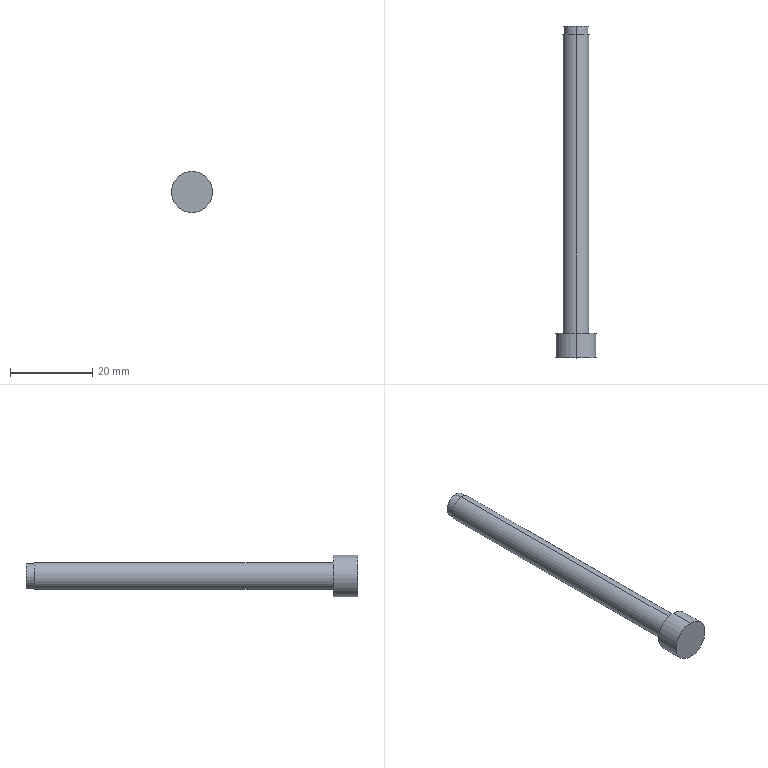Part | STEP file | 1 solid | 10 faces | box 10 x 80.703 x 10 mm | volume 2941 mm3 | cylinder 6 | plane 4 | commonest cylinder face diameters 6.03 x2 6.5 x2 10 x2
STEP:
#1=CARTESIAN_POINT('',(0.,0.,0.));
#2=DIRECTION('',(0.,0.,1.));
#3=DIRECTION('',(1.,0.,0.));
#4=AXIS2_PLACEMENT_3D('',#1,#2,#3);
#5=CARTESIAN_POINT('',(-85.927,-40.,121.58));
#6=VERTEX_POINT('',#5);
#7=CARTESIAN_POINT('',(-85.927,-40.,111.58));
#8=VERTEX_POINT('',#7);
#9=CARTESIAN_POINT('',(-85.927,-40.,116.58));
#10=DIRECTION('',(0.,1.,0.));
#11=DIRECTION('',(0.,0.,-1.));
#12=AXIS2_PLACEMENT_3D('',#9,#10,#11);
#13=CIRCLE('',#12,5.);
#14=CARTESIAN_POINT('',(-85.927,-50.,116.58));
#15=DIRECTION('',(0.,1.,0.));
#16=DIRECTION('',(0.,0.,1.));
#17=AXIS2_PLACEMENT_3D('',#14,#15,#16);
#18=CYLINDRICAL_SURFACE('',#17,5.);
#19=CARTESIAN_POINT('',(-3.142,10.));
#20=DIRECTION('',(1.,0.));
#21=VECTOR('',#20,1.);
#22=LINE('',#19,#21);
#23=(GEOMETRIC_REPRESENTATION_CONTEXT(2)PARAMETRIC_REPRESENTATION_CONTEXT()REPRESENTATION_CONTEXT('',''));
#24=DEFINITIONAL_REPRESENTATION('',(#22),#23);
#25=PCURVE('',#18,#24);
#26=CARTESIAN_POINT('',(-72.862,-40.,23.556));
#27=DIRECTION('',(0.,-1.,0.));
#28=DIRECTION('',(0.,0.,-1.));
#29=AXIS2_PLACEMENT_3D('',#26,#27,#28);
#30=PLANE('',#29);
#31=CARTESIAN_POINT('',(-88.024,-13.065));
#32=CARTESIAN_POINT('',(-88.024,-21.725));
#33=CARTESIAN_POINT('',(-95.524,-17.395));
#34=CARTESIAN_POINT('',(-103.024,-13.065));
#35=CARTESIAN_POINT('',(-95.524,-8.735));
#36=CARTESIAN_POINT('',(-88.024,-4.405));
#37=CARTESIAN_POINT('',(-88.024,-13.065));
#38=(BOUNDED_CURVE()B_SPLINE_CURVE(2,(#31,#32,#33,#34,#35,#36,#37),.UNSPECIFIED.,.T.,.F.)B_SPLINE_CURVE_WITH_KNOTS((1,2,2,2,2,1),(-2.094,0.,2.094,4.189,6.283,8.378),.UNSPECIFIED.)CURVE()GEOMETRIC_REPRESENTATION_ITEM()RATIONAL_B_SPLINE_CURVE((1.,0.5,1.,0.5,1.,0.5,1.))REPRESENTATION_ITEM(''));
#39=(GEOMETRIC_REPRESENTATION_CONTEXT(2)PARAMETRIC_REPRESENTATION_CONTEXT()REPRESENTATION_CONTEXT('',''));
#40=DEFINITIONAL_REPRESENTATION('',(#38),#39);
#41=PCURVE('',#30,#40);
#42=SURFACE_CURVE('',#13,(#25,#41),.PCURVE_S1.);
#43=EDGE_CURVE('',#6,#8,#42,.T.);
#44=ORIENTED_EDGE('',*,*,#43,.T.);
#45=CARTESIAN_POINT('',(-85.927,-34.,111.58));
#46=VERTEX_POINT('',#45);
#47=CARTESIAN_POINT('',(-85.927,-50.,111.58));
#48=DIRECTION('',(0.,1.,0.));
#49=VECTOR('',#48,1.);
#50=LINE('',#47,#49);
#51=CARTESIAN_POINT('',(3.142,0.));
#52=DIRECTION('',(0.,1.));
#53=VECTOR('',#52,1.);
#54=LINE('',#51,#53);
#55=(GEOMETRIC_REPRESENTATION_CONTEXT(2)PARAMETRIC_REPRESENTATION_CONTEXT()REPRESENTATION_CONTEXT('',''));
#56=DEFINITIONAL_REPRESENTATION('',(#54),#55);
#57=PCURVE('',#18,#56);
#58=CARTESIAN_POINT('',(-85.927,-50.,116.58));
#59=DIRECTION('',(0.,1.,0.));
#60=DIRECTION('',(0.,0.,1.));
#61=AXIS2_PLACEMENT_3D('',#58,#59,#60);
#62=CYLINDRICAL_SURFACE('',#61,5.);
#63=CARTESIAN_POINT('',(3.142,0.));
#64=DIRECTION('',(0.,1.));
#65=VECTOR('',#64,1.);
#66=LINE('',#63,#65);
#67=(GEOMETRIC_REPRESENTATION_CONTEXT(2)PARAMETRIC_REPRESENTATION_CONTEXT()REPRESENTATION_CONTEXT('',''));
#68=DEFINITIONAL_REPRESENTATION('',(#66),#67);
#69=PCURVE('',#62,#68);
#70=SURFACE_CURVE('',#50,(#57,#69),.PCURVE_S1.);
#71=EDGE_CURVE('',#8,#46,#70,.T.);
#72=ORIENTED_EDGE('',*,*,#71,.T.);
#73=CARTESIAN_POINT('',(-85.927,-34.,121.58));
#74=VERTEX_POINT('',#73);
#75=CARTESIAN_POINT('',(-85.927,-34.,116.58));
#76=DIRECTION('',(0.,-1.,0.));
#77=DIRECTION('',(0.,0.,-1.));
#78=AXIS2_PLACEMENT_3D('',#75,#76,#77);
#79=CIRCLE('',#78,5.);
#80=CARTESIAN_POINT('',(3.142,16.));
#81=DIRECTION('',(-1.,0.));
#82=VECTOR('',#81,1.);
#83=LINE('',#80,#82);
#84=(GEOMETRIC_REPRESENTATION_CONTEXT(2)PARAMETRIC_REPRESENTATION_CONTEXT()REPRESENTATION_CONTEXT('',''));
#85=DEFINITIONAL_REPRESENTATION('',(#83),#84);
#86=PCURVE('',#18,#85);
#87=CARTESIAN_POINT('',(-85.927,-34.,116.58));
#88=DIRECTION('',(0.,1.,0.));
#89=DIRECTION('',(0.,0.,1.));
#90=AXIS2_PLACEMENT_3D('',#87,#88,#89);
#91=PLANE('',#90);
#92=CARTESIAN_POINT('',(-5.,0.));
#93=CARTESIAN_POINT('',(-5.,8.66));
#94=CARTESIAN_POINT('',(2.5,4.33));
#95=CARTESIAN_POINT('',(10.,0.));
#96=CARTESIAN_POINT('',(2.5,-4.33));
#97=CARTESIAN_POINT('',(-5.,-8.66));
#98=CARTESIAN_POINT('',(-5.,0.));
#99=(BOUNDED_CURVE()B_SPLINE_CURVE(2,(#92,#93,#94,#95,#96,#97,#98),.UNSPECIFIED.,.T.,.F.)B_SPLINE_CURVE_WITH_KNOTS((1,2,2,2,2,1),(-2.094,0.,2.094,4.189,6.283,8.378),.UNSPECIFIED.)CURVE()GEOMETRIC_REPRESENTATION_ITEM()RATIONAL_B_SPLINE_CURVE((1.,0.5,1.,0.5,1.,0.5,1.))REPRESENTATION_ITEM(''));
#100=(GEOMETRIC_REPRESENTATION_CONTEXT(2)PARAMETRIC_REPRESENTATION_CONTEXT()REPRESENTATION_CONTEXT('',''));
#101=DEFINITIONAL_REPRESENTATION('',(#99),#100);
#102=PCURVE('',#91,#101);
#103=SURFACE_CURVE('',#79,(#86,#102),.PCURVE_S1.);
#104=EDGE_CURVE('',#46,#74,#103,.T.);
#105=ORIENTED_EDGE('',*,*,#104,.T.);
#106=CARTESIAN_POINT('',(-85.927,-50.,121.58));
#107=DIRECTION('',(0.,1.,0.));
#108=VECTOR('',#107,1.);
#109=LINE('',#106,#108);
#110=CARTESIAN_POINT('',(0.,0.));
#111=DIRECTION('',(0.,1.));
#112=VECTOR('',#111,1.);
#113=LINE('',#110,#112);
#114=(GEOMETRIC_REPRESENTATION_CONTEXT(2)PARAMETRIC_REPRESENTATION_CONTEXT()REPRESENTATION_CONTEXT('',''));
#115=DEFINITIONAL_REPRESENTATION('',(#113),#114);
#116=PCURVE('',#18,#115);
#117=CARTESIAN_POINT('',(6.283,0.));
#118=DIRECTION('',(0.,1.));
#119=VECTOR('',#118,1.);
#120=LINE('',#117,#119);
#121=(GEOMETRIC_REPRESENTATION_CONTEXT(2)PARAMETRIC_REPRESENTATION_CONTEXT()REPRESENTATION_CONTEXT('',''));
#122=DEFINITIONAL_REPRESENTATION('',(#120),#121);
#123=PCURVE('',#62,#122);
#124=SURFACE_CURVE('',#109,(#116,#123),.PCURVE_S1.);
#125=EDGE_CURVE('',#6,#74,#124,.T.);
#126=ORIENTED_EDGE('',*,*,#125,.F.);
#127=EDGE_LOOP('',(#44,#72,#105,#126));
#128=FACE_BOUND('',#127,.T.);
#129=ADVANCED_FACE('',(#128),#18,.T.);
#130=CARTESIAN_POINT('',(-85.927,38.693,119.83));
#131=VERTEX_POINT('',#130);
#132=CARTESIAN_POINT('',(-85.927,38.693,113.33));
#133=VERTEX_POINT('',#132);
#134=CARTESIAN_POINT('',(-85.927,38.693,116.58));
#135=DIRECTION('',(0.,1.,0.));
#136=DIRECTION('',(0.,0.,-1.));
#137=AXIS2_PLACEMENT_3D('',#134,#135,#136);
#138=CIRCLE('',#137,3.25);
#139=CARTESIAN_POINT('',(-85.927,40.703,116.58));
#140=DIRECTION('',(0.,-1.,0.));
#141=DIRECTION('',(0.,0.,-1.));
#142=AXIS2_PLACEMENT_3D('',#139,#140,#141);
#143=CYLINDRICAL_SURFACE('',#142,3.25);
#144=CARTESIAN_POINT('',(6.283,2.01));
#145=DIRECTION('',(-1.,0.));
#146=VECTOR('',#145,1.);
#147=LINE('',#144,#146);
#148=(GEOMETRIC_REPRESENTATION_CONTEXT(2)PARAMETRIC_REPRESENTATION_CONTEXT()REPRESENTATION_CONTEXT('',''));
#149=DEFINITIONAL_REPRESENTATION('',(#147),#148);
#150=PCURVE('',#143,#149);
#151=CARTESIAN_POINT('',(-111.957,38.693,127.032));
#152=DIRECTION('',(0.,-1.,0.));
#153=DIRECTION('',(0.,0.,-1.));
#154=AXIS2_PLACEMENT_3D('',#151,#152,#153);
#155=PLANE('',#154);
#156=CARTESIAN_POINT('',(13.702,26.029));
#157=CARTESIAN_POINT('',(13.702,20.4));
#158=CARTESIAN_POINT('',(8.827,23.215));
#159=CARTESIAN_POINT('',(3.952,26.029));
#160=CARTESIAN_POINT('',(8.827,28.844));
#161=CARTESIAN_POINT('',(13.702,31.659));
#162=CARTESIAN_POINT('',(13.702,26.029));
#163=(BOUNDED_CURVE()B_SPLINE_CURVE(2,(#156,#157,#158,#159,#160,#161,#162),.UNSPECIFIED.,.T.,.F.)B_SPLINE_CURVE_WITH_KNOTS((1,2,2,2,2,1),(-2.094,0.,2.094,4.189,6.283,8.378),.UNSPECIFIED.)CURVE()GEOMETRIC_REPRESENTATION_ITEM()RATIONAL_B_SPLINE_CURVE((1.,0.5,1.,0.5,1.,0.5,1.))REPRESENTATION_ITEM(''));
#164=(GEOMETRIC_REPRESENTATION_CONTEXT(2)PARAMETRIC_REPRESENTATION_CONTEXT()REPRESENTATION_CONTEXT('',''));
#165=DEFINITIONAL_REPRESENTATION('',(#163),#164);
#166=PCURVE('',#155,#165);
#167=SURFACE_CURVE('',#138,(#150,#166),.PCURVE_S1.);
#168=EDGE_CURVE('',#131,#133,#167,.T.);
#169=ORIENTED_EDGE('',*,*,#168,.F.);
#170=CARTESIAN_POINT('',(-85.927,-34.,119.83));
#171=VERTEX_POINT('',#170);
#172=CARTESIAN_POINT('',(-85.927,40.703,119.83));
#173=DIRECTION('',(0.,-1.,0.));
#174=VECTOR('',#173,1.);
#175=LINE('',#172,#174);
#176=CARTESIAN_POINT('',(3.142,0.));
#177=DIRECTION('',(0.,1.));
#178=VECTOR('',#177,1.);
#179=LINE('',#176,#178);
#180=(GEOMETRIC_REPRESENTATION_CONTEXT(2)PARAMETRIC_REPRESENTATION_CONTEXT()REPRESENTATION_CONTEXT('',''));
#181=DEFINITIONAL_REPRESENTATION('',(#179),#180);
#182=PCURVE('',#143,#181);
#183=CARTESIAN_POINT('',(-85.927,40.703,116.58));
#184=DIRECTION('',(0.,-1.,0.));
#185=DIRECTION('',(0.,0.,-1.));
#186=AXIS2_PLACEMENT_3D('',#183,#184,#185);
#187=CYLINDRICAL_SURFACE('',#186,3.25);
#188=CARTESIAN_POINT('',(3.142,0.));
#189=DIRECTION('',(0.,1.));
#190=VECTOR('',#189,1.);
#191=LINE('',#188,#190);
#192=(GEOMETRIC_REPRESENTATION_CONTEXT(2)PARAMETRIC_REPRESENTATION_CONTEXT()REPRESENTATION_CONTEXT('',''));
#193=DEFINITIONAL_REPRESENTATION('',(#191),#192);
#194=PCURVE('',#187,#193);
#195=SURFACE_CURVE('',#175,(#182,#194),.PCURVE_S1.);
#196=EDGE_CURVE('',#131,#171,#195,.T.);
#197=ORIENTED_EDGE('',*,*,#196,.T.);
#198=CARTESIAN_POINT('',(-85.927,-34.,113.33));
#199=VERTEX_POINT('',#198);
#200=CARTESIAN_POINT('',(-85.927,-34.,116.58));
#201=DIRECTION('',(0.,-1.,0.));
#202=DIRECTION('',(0.,0.,1.));
#203=AXIS2_PLACEMENT_3D('',#200,#201,#202);
#204=CIRCLE('',#203,3.25);
#205=CARTESIAN_POINT('',(-3.142,74.703));
#206=DIRECTION('',(1.,0.));
#207=VECTOR('',#206,1.);
#208=LINE('',#205,#207);
#209=(GEOMETRIC_REPRESENTATION_CONTEXT(2)PARAMETRIC_REPRESENTATION_CONTEXT()REPRESENTATION_CONTEXT('',''));
#210=DEFINITIONAL_REPRESENTATION('',(#208),#209);
#211=PCURVE('',#143,#210);
#212=CARTESIAN_POINT('',(3.25,0.));
#213=CARTESIAN_POINT('',(3.25,-5.629));
#214=CARTESIAN_POINT('',(-1.625,-2.815));
#215=CARTESIAN_POINT('',(-6.5,0.));
#216=CARTESIAN_POINT('',(-1.625,2.815));
#217=CARTESIAN_POINT('',(3.25,5.629));
#218=CARTESIAN_POINT('',(3.25,0.));
#219=(BOUNDED_CURVE()B_SPLINE_CURVE(2,(#212,#213,#214,#215,#216,#217,#218),.UNSPECIFIED.,.T.,.F.)B_SPLINE_CURVE_WITH_KNOTS((1,2,2,2,2,1),(-2.094,0.,2.094,4.189,6.283,8.378),.UNSPECIFIED.)CURVE()GEOMETRIC_REPRESENTATION_ITEM()RATIONAL_B_SPLINE_CURVE((1.,0.5,1.,0.5,1.,0.5,1.))REPRESENTATION_ITEM(''));
#220=(GEOMETRIC_REPRESENTATION_CONTEXT(2)PARAMETRIC_REPRESENTATION_CONTEXT()REPRESENTATION_CONTEXT('',''));
#221=DEFINITIONAL_REPRESENTATION('',(#219),#220);
#222=PCURVE('',#91,#221);
#223=SURFACE_CURVE('',#204,(#211,#222),.PCURVE_S1.);
#224=EDGE_CURVE('',#199,#171,#223,.T.);
#225=ORIENTED_EDGE('',*,*,#224,.F.);
#226=CARTESIAN_POINT('',(-85.927,40.703,113.33));
#227=DIRECTION('',(0.,-1.,0.));
#228=VECTOR('',#227,1.);
#229=LINE('',#226,#228);
#230=CARTESIAN_POINT('',(0.,0.));
#231=DIRECTION('',(0.,1.));
#232=VECTOR('',#231,1.);
#233=LINE('',#230,#232);
#234=(GEOMETRIC_REPRESENTATION_CONTEXT(2)PARAMETRIC_REPRESENTATION_CONTEXT()REPRESENTATION_CONTEXT('',''));
#235=DEFINITIONAL_REPRESENTATION('',(#233),#234);
#236=PCURVE('',#143,#235);
#237=CARTESIAN_POINT('',(6.283,0.));
#238=DIRECTION('',(0.,1.));
#239=VECTOR('',#238,1.);
#240=LINE('',#237,#239);
#241=(GEOMETRIC_REPRESENTATION_CONTEXT(2)PARAMETRIC_REPRESENTATION_CONTEXT()REPRESENTATION_CONTEXT('',''));
#242=DEFINITIONAL_REPRESENTATION('',(#240),#241);
#243=PCURVE('',#187,#242);
#244=SURFACE_CURVE('',#229,(#236,#243),.PCURVE_S1.);
#245=EDGE_CURVE('',#133,#199,#244,.T.);
#246=ORIENTED_EDGE('',*,*,#245,.F.);
#247=EDGE_LOOP('',(#169,#197,#225,#246));
#248=FACE_BOUND('',#247,.T.);
#249=ADVANCED_FACE('',(#248),#143,.T.);
#250=CARTESIAN_POINT('',(-85.927,40.703,119.595));
#251=VERTEX_POINT('',#250);
#252=CARTESIAN_POINT('',(-85.927,40.703,113.565));
#253=VERTEX_POINT('',#252);
#254=CARTESIAN_POINT('',(-85.927,40.703,116.58));
#255=DIRECTION('',(0.,1.,0.));
#256=DIRECTION('',(0.,0.,1.));
#257=AXIS2_PLACEMENT_3D('',#254,#255,#256);
#258=CIRCLE('',#257,3.015);
#259=CARTESIAN_POINT('',(-85.927,41.708,116.58));
#260=DIRECTION('',(0.,-1.,0.));
#261=DIRECTION('',(0.,0.,-1.));
#262=AXIS2_PLACEMENT_3D('',#259,#260,#261);
#263=CYLINDRICAL_SURFACE('',#262,3.015);
#264=CARTESIAN_POINT('',(3.142,1.005));
#265=DIRECTION('',(-1.,0.));
#266=VECTOR('',#265,1.);
#267=LINE('',#264,#266);
#268=(GEOMETRIC_REPRESENTATION_CONTEXT(2)PARAMETRIC_REPRESENTATION_CONTEXT()REPRESENTATION_CONTEXT('',''));
#269=DEFINITIONAL_REPRESENTATION('',(#267),#268);
#270=PCURVE('',#263,#269);
#271=CARTESIAN_POINT('',(-85.927,40.703,116.58));
#272=DIRECTION('',(0.,1.,0.));
#273=DIRECTION('',(0.,0.,1.));
#274=AXIS2_PLACEMENT_3D('',#271,#272,#273);
#275=PLANE('',#274);
#276=CARTESIAN_POINT('',(0.,0.));
#277=DIRECTION('',(1.,0.));
#278=AXIS2_PLACEMENT_2D('',#276,#277);
#279=CIRCLE('',#278,3.015);
#280=(GEOMETRIC_REPRESENTATION_CONTEXT(2)PARAMETRIC_REPRESENTATION_CONTEXT()REPRESENTATION_CONTEXT('',''));
#281=DEFINITIONAL_REPRESENTATION('',(#279),#280);
#282=PCURVE('',#275,#281);
#283=SURFACE_CURVE('',#258,(#270,#282),.PCURVE_S1.);
#284=EDGE_CURVE('',#251,#253,#283,.T.);
#285=ORIENTED_EDGE('',*,*,#284,.F.);
#286=CARTESIAN_POINT('',(-85.927,38.693,119.595));
#287=VERTEX_POINT('',#286);
#288=CARTESIAN_POINT('',(-85.927,41.708,119.595));
#289=DIRECTION('',(0.,-1.,0.));
#290=VECTOR('',#289,1.);
#291=LINE('',#288,#290);
#292=CARTESIAN_POINT('',(3.142,0.));
#293=DIRECTION('',(0.,1.));
#294=VECTOR('',#293,1.);
#295=LINE('',#292,#294);
#296=(GEOMETRIC_REPRESENTATION_CONTEXT(2)PARAMETRIC_REPRESENTATION_CONTEXT()REPRESENTATION_CONTEXT('',''));
#297=DEFINITIONAL_REPRESENTATION('',(#295),#296);
#298=PCURVE('',#263,#297);
#299=CARTESIAN_POINT('',(-85.927,41.708,116.58));
#300=DIRECTION('',(0.,-1.,0.));
#301=DIRECTION('',(0.,0.,-1.));
#302=AXIS2_PLACEMENT_3D('',#299,#300,#301);
#303=CYLINDRICAL_SURFACE('',#302,3.015);
#304=CARTESIAN_POINT('',(3.142,0.));
#305=DIRECTION('',(0.,1.));
#306=VECTOR('',#305,1.);
#307=LINE('',#304,#306);
#308=(GEOMETRIC_REPRESENTATION_CONTEXT(2)PARAMETRIC_REPRESENTATION_CONTEXT()REPRESENTATION_CONTEXT('',''));
#309=DEFINITIONAL_REPRESENTATION('',(#307),#308);
#310=PCURVE('',#303,#309);
#311=SURFACE_CURVE('',#291,(#298,#310),.PCURVE_S1.);
#312=EDGE_CURVE('',#251,#287,#311,.T.);
#313=ORIENTED_EDGE('',*,*,#312,.T.);
#314=CARTESIAN_POINT('',(-85.927,38.693,113.565));
#315=VERTEX_POINT('',#314);
#316=CARTESIAN_POINT('',(-85.927,38.693,116.58));
#317=DIRECTION('',(0.,-1.,0.));
#318=DIRECTION('',(0.,0.,-1.));
#319=AXIS2_PLACEMENT_3D('',#316,#317,#318);
#320=CIRCLE('',#319,3.015);
#321=CARTESIAN_POINT('',(0.,3.015));
#322=DIRECTION('',(1.,0.));
#323=VECTOR('',#322,1.);
#324=LINE('',#321,#323);
#325=(GEOMETRIC_REPRESENTATION_CONTEXT(2)PARAMETRIC_REPRESENTATION_CONTEXT()REPRESENTATION_CONTEXT('',''));
#326=DEFINITIONAL_REPRESENTATION('',(#324),#325);
#327=PCURVE('',#263,#326);
#328=CARTESIAN_POINT('',(10.452,26.029));
#329=DIRECTION('',(1.,0.));
#330=AXIS2_PLACEMENT_2D('',#328,#329);
#331=CIRCLE('',#330,3.015);
#332=(GEOMETRIC_REPRESENTATION_CONTEXT(2)PARAMETRIC_REPRESENTATION_CONTEXT()REPRESENTATION_CONTEXT('',''));
#333=DEFINITIONAL_REPRESENTATION('',(#331),#332);
#334=PCURVE('',#155,#333);
#335=SURFACE_CURVE('',#320,(#327,#334),.PCURVE_S1.);
#336=EDGE_CURVE('',#315,#287,#335,.T.);
#337=ORIENTED_EDGE('',*,*,#336,.F.);
#338=CARTESIAN_POINT('',(-85.927,41.708,113.565));
#339=DIRECTION('',(0.,-1.,0.));
#340=VECTOR('',#339,1.);
#341=LINE('',#338,#340);
#342=CARTESIAN_POINT('',(0.,0.));
#343=DIRECTION('',(0.,1.));
#344=VECTOR('',#343,1.);
#345=LINE('',#342,#344);
#346=(GEOMETRIC_REPRESENTATION_CONTEXT(2)PARAMETRIC_REPRESENTATION_CONTEXT()REPRESENTATION_CONTEXT('',''));
#347=DEFINITIONAL_REPRESENTATION('',(#345),#346);
#348=PCURVE('',#263,#347);
#349=CARTESIAN_POINT('',(6.283,0.));
#350=DIRECTION('',(0.,1.));
#351=VECTOR('',#350,1.);
#352=LINE('',#349,#351);
#353=(GEOMETRIC_REPRESENTATION_CONTEXT(2)PARAMETRIC_REPRESENTATION_CONTEXT()REPRESENTATION_CONTEXT('',''));
#354=DEFINITIONAL_REPRESENTATION('',(#352),#353);
#355=PCURVE('',#303,#354);
#356=SURFACE_CURVE('',#341,(#348,#355),.PCURVE_S1.);
#357=EDGE_CURVE('',#253,#315,#356,.T.);
#358=ORIENTED_EDGE('',*,*,#357,.F.);
#359=EDGE_LOOP('',(#285,#313,#337,#358));
#360=FACE_BOUND('',#359,.T.);
#361=ADVANCED_FACE('',(#360),#263,.T.);
#362=CARTESIAN_POINT('',(-85.927,38.693,116.58));
#363=DIRECTION('',(0.,1.,0.));
#364=DIRECTION('',(0.,0.,-1.));
#365=AXIS2_PLACEMENT_3D('',#362,#363,#364);
#366=CIRCLE('',#365,3.25);
#367=CARTESIAN_POINT('',(13.702,26.029));
#368=CARTESIAN_POINT('',(13.702,20.4));
#369=CARTESIAN_POINT('',(8.827,23.215));
#370=CARTESIAN_POINT('',(3.952,26.029));
#371=CARTESIAN_POINT('',(8.827,28.844));
#372=CARTESIAN_POINT('',(13.702,31.659));
#373=CARTESIAN_POINT('',(13.702,26.029));
#374=(BOUNDED_CURVE()B_SPLINE_CURVE(2,(#367,#368,#369,#370,#371,#372,#373),.UNSPECIFIED.,.T.,.F.)B_SPLINE_CURVE_WITH_KNOTS((1,2,2,2,2,1),(-2.094,0.,2.094,4.189,6.283,8.378),.UNSPECIFIED.)CURVE()GEOMETRIC_REPRESENTATION_ITEM()RATIONAL_B_SPLINE_CURVE((1.,0.5,1.,0.5,1.,0.5,1.))REPRESENTATION_ITEM(''));
#375=(GEOMETRIC_REPRESENTATION_CONTEXT(2)PARAMETRIC_REPRESENTATION_CONTEXT()REPRESENTATION_CONTEXT('',''));
#376=DEFINITIONAL_REPRESENTATION('',(#374),#375);
#377=PCURVE('',#155,#376);
#378=CARTESIAN_POINT('',(6.283,2.01));
#379=DIRECTION('',(-1.,0.));
#380=VECTOR('',#379,1.);
#381=LINE('',#378,#380);
#382=(GEOMETRIC_REPRESENTATION_CONTEXT(2)PARAMETRIC_REPRESENTATION_CONTEXT()REPRESENTATION_CONTEXT('',''));
#383=DEFINITIONAL_REPRESENTATION('',(#381),#382);
#384=PCURVE('',#187,#383);
#385=SURFACE_CURVE('',#366,(#377,#384),.PCURVE_S1.);
#386=EDGE_CURVE('',#133,#131,#385,.T.);
#387=ORIENTED_EDGE('',*,*,#386,.T.);
#388=ORIENTED_EDGE('',*,*,#168,.T.);
#389=EDGE_LOOP('',(#387,#388));
#390=FACE_BOUND('',#389,.T.);
#391=ORIENTED_EDGE('',*,*,#336,.T.);
#392=CARTESIAN_POINT('',(-85.927,38.693,116.58));
#393=DIRECTION('',(0.,-1.,0.));
#394=DIRECTION('',(0.,0.,-1.));
#395=AXIS2_PLACEMENT_3D('',#392,#393,#394);
#396=CIRCLE('',#395,3.015);
#397=CARTESIAN_POINT('',(10.452,26.029));
#398=DIRECTION('',(1.,0.));
#399=AXIS2_PLACEMENT_2D('',#397,#398);
#400=CIRCLE('',#399,3.015);
#401=(GEOMETRIC_REPRESENTATION_CONTEXT(2)PARAMETRIC_REPRESENTATION_CONTEXT()REPRESENTATION_CONTEXT('',''));
#402=DEFINITIONAL_REPRESENTATION('',(#400),#401);
#403=PCURVE('',#155,#402);
#404=CARTESIAN_POINT('',(0.,3.015));
#405=DIRECTION('',(1.,0.));
#406=VECTOR('',#405,1.);
#407=LINE('',#404,#406);
#408=(GEOMETRIC_REPRESENTATION_CONTEXT(2)PARAMETRIC_REPRESENTATION_CONTEXT()REPRESENTATION_CONTEXT('',''));
#409=DEFINITIONAL_REPRESENTATION('',(#407),#408);
#410=PCURVE('',#303,#409);
#411=SURFACE_CURVE('',#396,(#403,#410),.PCURVE_S1.);
#412=EDGE_CURVE('',#287,#315,#411,.T.);
#413=ORIENTED_EDGE('',*,*,#412,.T.);
#414=EDGE_LOOP('',(#391,#413));
#415=FACE_BOUND('',#414,.T.);
#416=ADVANCED_FACE('',(#390,#415),#155,.F.);
#417=ORIENTED_EDGE('',*,*,#312,.F.);
#418=CARTESIAN_POINT('',(-85.927,40.703,116.58));
#419=DIRECTION('',(0.,1.,0.));
#420=DIRECTION('',(0.,0.,1.));
#421=AXIS2_PLACEMENT_3D('',#418,#419,#420);
#422=CIRCLE('',#421,3.015);
#423=CARTESIAN_POINT('',(9.425,1.005));
#424=DIRECTION('',(-1.,0.));
#425=VECTOR('',#424,1.);
#426=LINE('',#423,#425);
#427=(GEOMETRIC_REPRESENTATION_CONTEXT(2)PARAMETRIC_REPRESENTATION_CONTEXT()REPRESENTATION_CONTEXT('',''));
#428=DEFINITIONAL_REPRESENTATION('',(#426),#427);
#429=PCURVE('',#303,#428);
#430=CARTESIAN_POINT('',(0.,0.));
#431=DIRECTION('',(1.,0.));
#432=AXIS2_PLACEMENT_2D('',#430,#431);
#433=CIRCLE('',#432,3.015);
#434=(GEOMETRIC_REPRESENTATION_CONTEXT(2)PARAMETRIC_REPRESENTATION_CONTEXT()REPRESENTATION_CONTEXT('',''));
#435=DEFINITIONAL_REPRESENTATION('',(#433),#434);
#436=PCURVE('',#275,#435);
#437=SURFACE_CURVE('',#422,(#429,#436),.PCURVE_S1.);
#438=EDGE_CURVE('',#253,#251,#437,.T.);
#439=ORIENTED_EDGE('',*,*,#438,.F.);
#440=ORIENTED_EDGE('',*,*,#357,.T.);
#441=ORIENTED_EDGE('',*,*,#412,.F.);
#442=EDGE_LOOP('',(#417,#439,#440,#441));
#443=FACE_BOUND('',#442,.T.);
#444=ADVANCED_FACE('',(#443),#303,.T.);
#445=ORIENTED_EDGE('',*,*,#196,.F.);
#446=ORIENTED_EDGE('',*,*,#386,.F.);
#447=ORIENTED_EDGE('',*,*,#245,.T.);
#448=CARTESIAN_POINT('',(-85.927,-34.,116.58));
#449=DIRECTION('',(0.,-1.,0.));
#450=DIRECTION('',(0.,0.,1.));
#451=AXIS2_PLACEMENT_3D('',#448,#449,#450);
#452=CIRCLE('',#451,3.25);
#453=CARTESIAN_POINT('',(3.142,74.703));
#454=DIRECTION('',(1.,0.));
#455=VECTOR('',#454,1.);
#456=LINE('',#453,#455);
#457=(GEOMETRIC_REPRESENTATION_CONTEXT(2)PARAMETRIC_REPRESENTATION_CONTEXT()REPRESENTATION_CONTEXT('',''));
#458=DEFINITIONAL_REPRESENTATION('',(#456),#457);
#459=PCURVE('',#187,#458);
#460=CARTESIAN_POINT('',(3.25,0.));
#461=CARTESIAN_POINT('',(3.25,-5.629));
#462=CARTESIAN_POINT('',(-1.625,-2.815));
#463=CARTESIAN_POINT('',(-6.5,0.));
#464=CARTESIAN_POINT('',(-1.625,2.815));
#465=CARTESIAN_POINT('',(3.25,5.629));
#466=CARTESIAN_POINT('',(3.25,0.));
#467=(BOUNDED_CURVE()B_SPLINE_CURVE(2,(#460,#461,#462,#463,#464,#465,#466),.UNSPECIFIED.,.T.,.F.)B_SPLINE_CURVE_WITH_KNOTS((1,2,2,2,2,1),(-2.094,0.,2.094,4.189,6.283,8.378),.UNSPECIFIED.)CURVE()GEOMETRIC_REPRESENTATION_ITEM()RATIONAL_B_SPLINE_CURVE((1.,0.5,1.,0.5,1.,0.5,1.))REPRESENTATION_ITEM(''));
#468=(GEOMETRIC_REPRESENTATION_CONTEXT(2)PARAMETRIC_REPRESENTATION_CONTEXT()REPRESENTATION_CONTEXT('',''));
#469=DEFINITIONAL_REPRESENTATION('',(#467),#468);
#470=PCURVE('',#91,#469);
#471=SURFACE_CURVE('',#452,(#459,#470),.PCURVE_S1.);
#472=EDGE_CURVE('',#171,#199,#471,.T.);
#473=ORIENTED_EDGE('',*,*,#472,.F.);
#474=EDGE_LOOP('',(#445,#446,#447,#473));
#475=FACE_BOUND('',#474,.T.);
#476=ADVANCED_FACE('',(#475),#187,.T.);
#477=ORIENTED_EDGE('',*,*,#438,.T.);
#478=ORIENTED_EDGE('',*,*,#284,.T.);
#479=EDGE_LOOP('',(#477,#478));
#480=FACE_BOUND('',#479,.T.);
#481=ADVANCED_FACE('',(#480),#275,.T.);
#482=ORIENTED_EDGE('',*,*,#224,.T.);
#483=ORIENTED_EDGE('',*,*,#472,.T.);
#484=EDGE_LOOP('',(#482,#483));
#485=FACE_BOUND('',#484,.T.);
#486=CARTESIAN_POINT('',(-85.927,-34.,116.58));
#487=DIRECTION('',(0.,-1.,0.));
#488=DIRECTION('',(0.,0.,-1.));
#489=AXIS2_PLACEMENT_3D('',#486,#487,#488);
#490=CIRCLE('',#489,5.);
#491=CARTESIAN_POINT('',(-5.,0.));
#492=CARTESIAN_POINT('',(-5.,8.66));
#493=CARTESIAN_POINT('',(2.5,4.33));
#494=CARTESIAN_POINT('',(10.,0.));
#495=CARTESIAN_POINT('',(2.5,-4.33));
#496=CARTESIAN_POINT('',(-5.,-8.66));
#497=CARTESIAN_POINT('',(-5.,0.));
#498=(BOUNDED_CURVE()B_SPLINE_CURVE(2,(#491,#492,#493,#494,#495,#496,#497),.UNSPECIFIED.,.T.,.F.)B_SPLINE_CURVE_WITH_KNOTS((1,2,2,2,2,1),(-2.094,0.,2.094,4.189,6.283,8.378),.UNSPECIFIED.)CURVE()GEOMETRIC_REPRESENTATION_ITEM()RATIONAL_B_SPLINE_CURVE((1.,0.5,1.,0.5,1.,0.5,1.))REPRESENTATION_ITEM(''));
#499=(GEOMETRIC_REPRESENTATION_CONTEXT(2)PARAMETRIC_REPRESENTATION_CONTEXT()REPRESENTATION_CONTEXT('',''));
#500=DEFINITIONAL_REPRESENTATION('',(#498),#499);
#501=PCURVE('',#91,#500);
#502=CARTESIAN_POINT('',(9.425,16.));
#503=DIRECTION('',(-1.,0.));
#504=VECTOR('',#503,1.);
#505=LINE('',#502,#504);
#506=(GEOMETRIC_REPRESENTATION_CONTEXT(2)PARAMETRIC_REPRESENTATION_CONTEXT()REPRESENTATION_CONTEXT('',''));
#507=DEFINITIONAL_REPRESENTATION('',(#505),#506);
#508=PCURVE('',#62,#507);
#509=SURFACE_CURVE('',#490,(#501,#508),.PCURVE_S1.);
#510=EDGE_CURVE('',#74,#46,#509,.T.);
#511=ORIENTED_EDGE('',*,*,#510,.F.);
#512=ORIENTED_EDGE('',*,*,#104,.F.);
#513=EDGE_LOOP('',(#511,#512));
#514=FACE_BOUND('',#513,.T.);
#515=ADVANCED_FACE('',(#485,#514),#91,.T.);
#516=ORIENTED_EDGE('',*,*,#71,.F.);
#517=CARTESIAN_POINT('',(-85.927,-40.,116.58));
#518=DIRECTION('',(0.,1.,0.));
#519=DIRECTION('',(0.,0.,-1.));
#520=AXIS2_PLACEMENT_3D('',#517,#518,#519);
#521=CIRCLE('',#520,5.);
#522=CARTESIAN_POINT('',(3.142,10.));
#523=DIRECTION('',(1.,0.));
#524=VECTOR('',#523,1.);
#525=LINE('',#522,#524);
#526=(GEOMETRIC_REPRESENTATION_CONTEXT(2)PARAMETRIC_REPRESENTATION_CONTEXT()REPRESENTATION_CONTEXT('',''));
#527=DEFINITIONAL_REPRESENTATION('',(#525),#526);
#528=PCURVE('',#62,#527);
#529=CARTESIAN_POINT('',(-88.024,-13.065));
#530=CARTESIAN_POINT('',(-88.024,-21.725));
#531=CARTESIAN_POINT('',(-95.524,-17.395));
#532=CARTESIAN_POINT('',(-103.024,-13.065));
#533=CARTESIAN_POINT('',(-95.524,-8.735));
#534=CARTESIAN_POINT('',(-88.024,-4.405));
#535=CARTESIAN_POINT('',(-88.024,-13.065));
#536=(BOUNDED_CURVE()B_SPLINE_CURVE(2,(#529,#530,#531,#532,#533,#534,#535),.UNSPECIFIED.,.T.,.F.)B_SPLINE_CURVE_WITH_KNOTS((1,2,2,2,2,1),(-2.094,0.,2.094,4.189,6.283,8.378),.UNSPECIFIED.)CURVE()GEOMETRIC_REPRESENTATION_ITEM()RATIONAL_B_SPLINE_CURVE((1.,0.5,1.,0.5,1.,0.5,1.))REPRESENTATION_ITEM(''));
#537=(GEOMETRIC_REPRESENTATION_CONTEXT(2)PARAMETRIC_REPRESENTATION_CONTEXT()REPRESENTATION_CONTEXT('',''));
#538=DEFINITIONAL_REPRESENTATION('',(#536),#537);
#539=PCURVE('',#30,#538);
#540=SURFACE_CURVE('',#521,(#528,#539),.PCURVE_S1.);
#541=EDGE_CURVE('',#8,#6,#540,.T.);
#542=ORIENTED_EDGE('',*,*,#541,.T.);
#543=ORIENTED_EDGE('',*,*,#125,.T.);
#544=ORIENTED_EDGE('',*,*,#510,.T.);
#545=EDGE_LOOP('',(#516,#542,#543,#544));
#546=FACE_BOUND('',#545,.T.);
#547=ADVANCED_FACE('',(#546),#62,.T.);
#548=ORIENTED_EDGE('',*,*,#43,.F.);
#549=ORIENTED_EDGE('',*,*,#541,.F.);
#550=EDGE_LOOP('',(#548,#549));
#551=FACE_BOUND('',#550,.T.);
#552=ADVANCED_FACE('',(#551),#30,.T.);
#553=CLOSED_SHELL('',(#129,#249,#361,#416,#444,#476,#481,#515,#547,#552));
#554=MANIFOLD_SOLID_BREP('',#553);
#555=(LENGTH_UNIT()NAMED_UNIT(*)SI_UNIT(.MILLI.,.METRE.));
#556=UNCERTAINTY_MEASURE_WITH_UNIT(LENGTH_MEASURE(0.0000001),#555,'','');
#557=(NAMED_UNIT(*)PLANE_ANGLE_UNIT()SI_UNIT($,.RADIAN.));
#558=(NAMED_UNIT(*)SI_UNIT($,.STERADIAN.)SOLID_ANGLE_UNIT());
#559=(GEOMETRIC_REPRESENTATION_CONTEXT(3)GLOBAL_UNCERTAINTY_ASSIGNED_CONTEXT((#556))GLOBAL_UNIT_ASSIGNED_CONTEXT((#555,#557,#558))REPRESENTATION_CONTEXT('',''));
#560=ADVANCED_BREP_SHAPE_REPRESENTATION('',(#4,#554),#559);